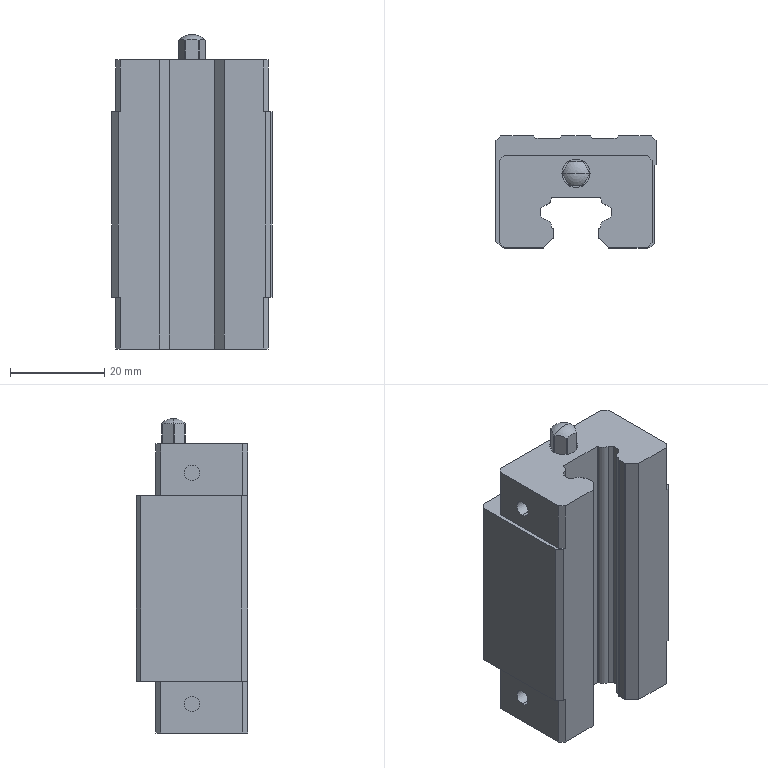Part | SolidWorks | features BaseBody 1 | 1 solid | 139 faces | box 34 x 23.7 x 66.7 mm | volume 36765 mm3 | plane 70 | cylinder 51 | cone 16 | torus 2 | commonest cylinder face diameters 0.8 x8 3.242 x8 3.3 x8 0.4 x7 1 x4 3.24 x4